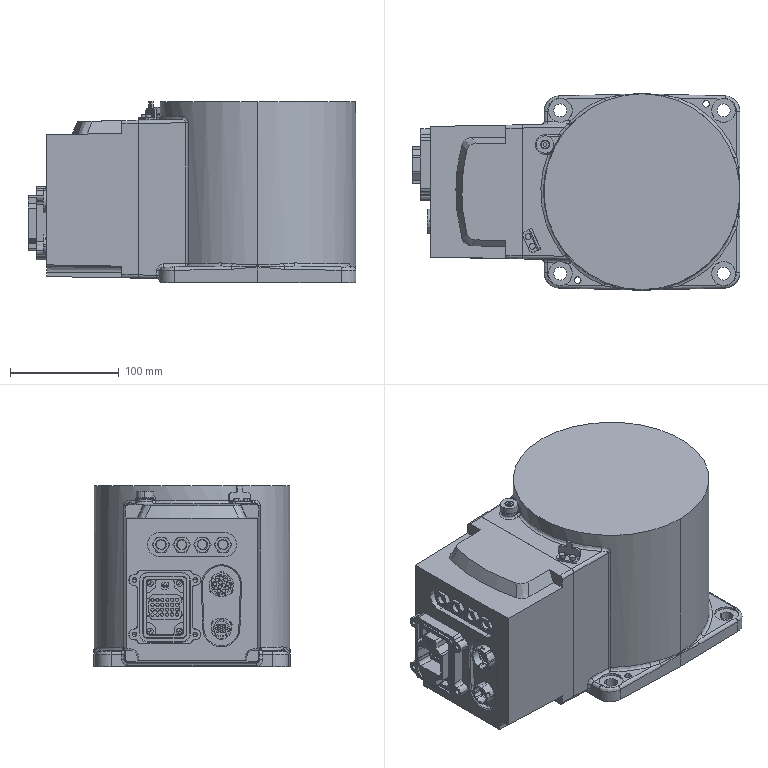Part | STEP file | ASND-0110-IRB120_3-58_IRC5_Base_rev0 | 15 solids | 1413 faces | box 301.2 x 180.524 x 166.334 mm | volume 6215073 mm3 | plane 747 | cylinder 410 | cone 116 | torus 80 | spline 58 | sphere 2 | commonest cylinder face diameters 3 x54 3.3 x54 6 x40 3.1 x24 2.083 x20 5.5 x12